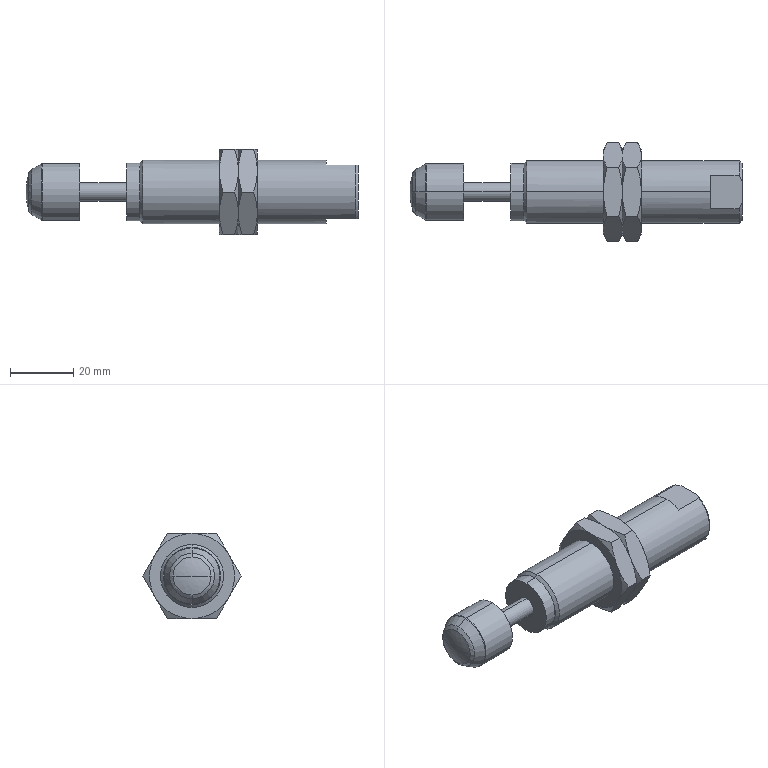Part | STEP file | 3 solids | 83 faces | box 105.2 x 31.177 x 27 mm | volume 31063 mm3 | cone 38 | plane 25 | cylinder 14 | spline 6 | commonest cylinder face diameters 18.376 x4 6 x2 6.8 x2 18 x2 18.2 x2 20 x2